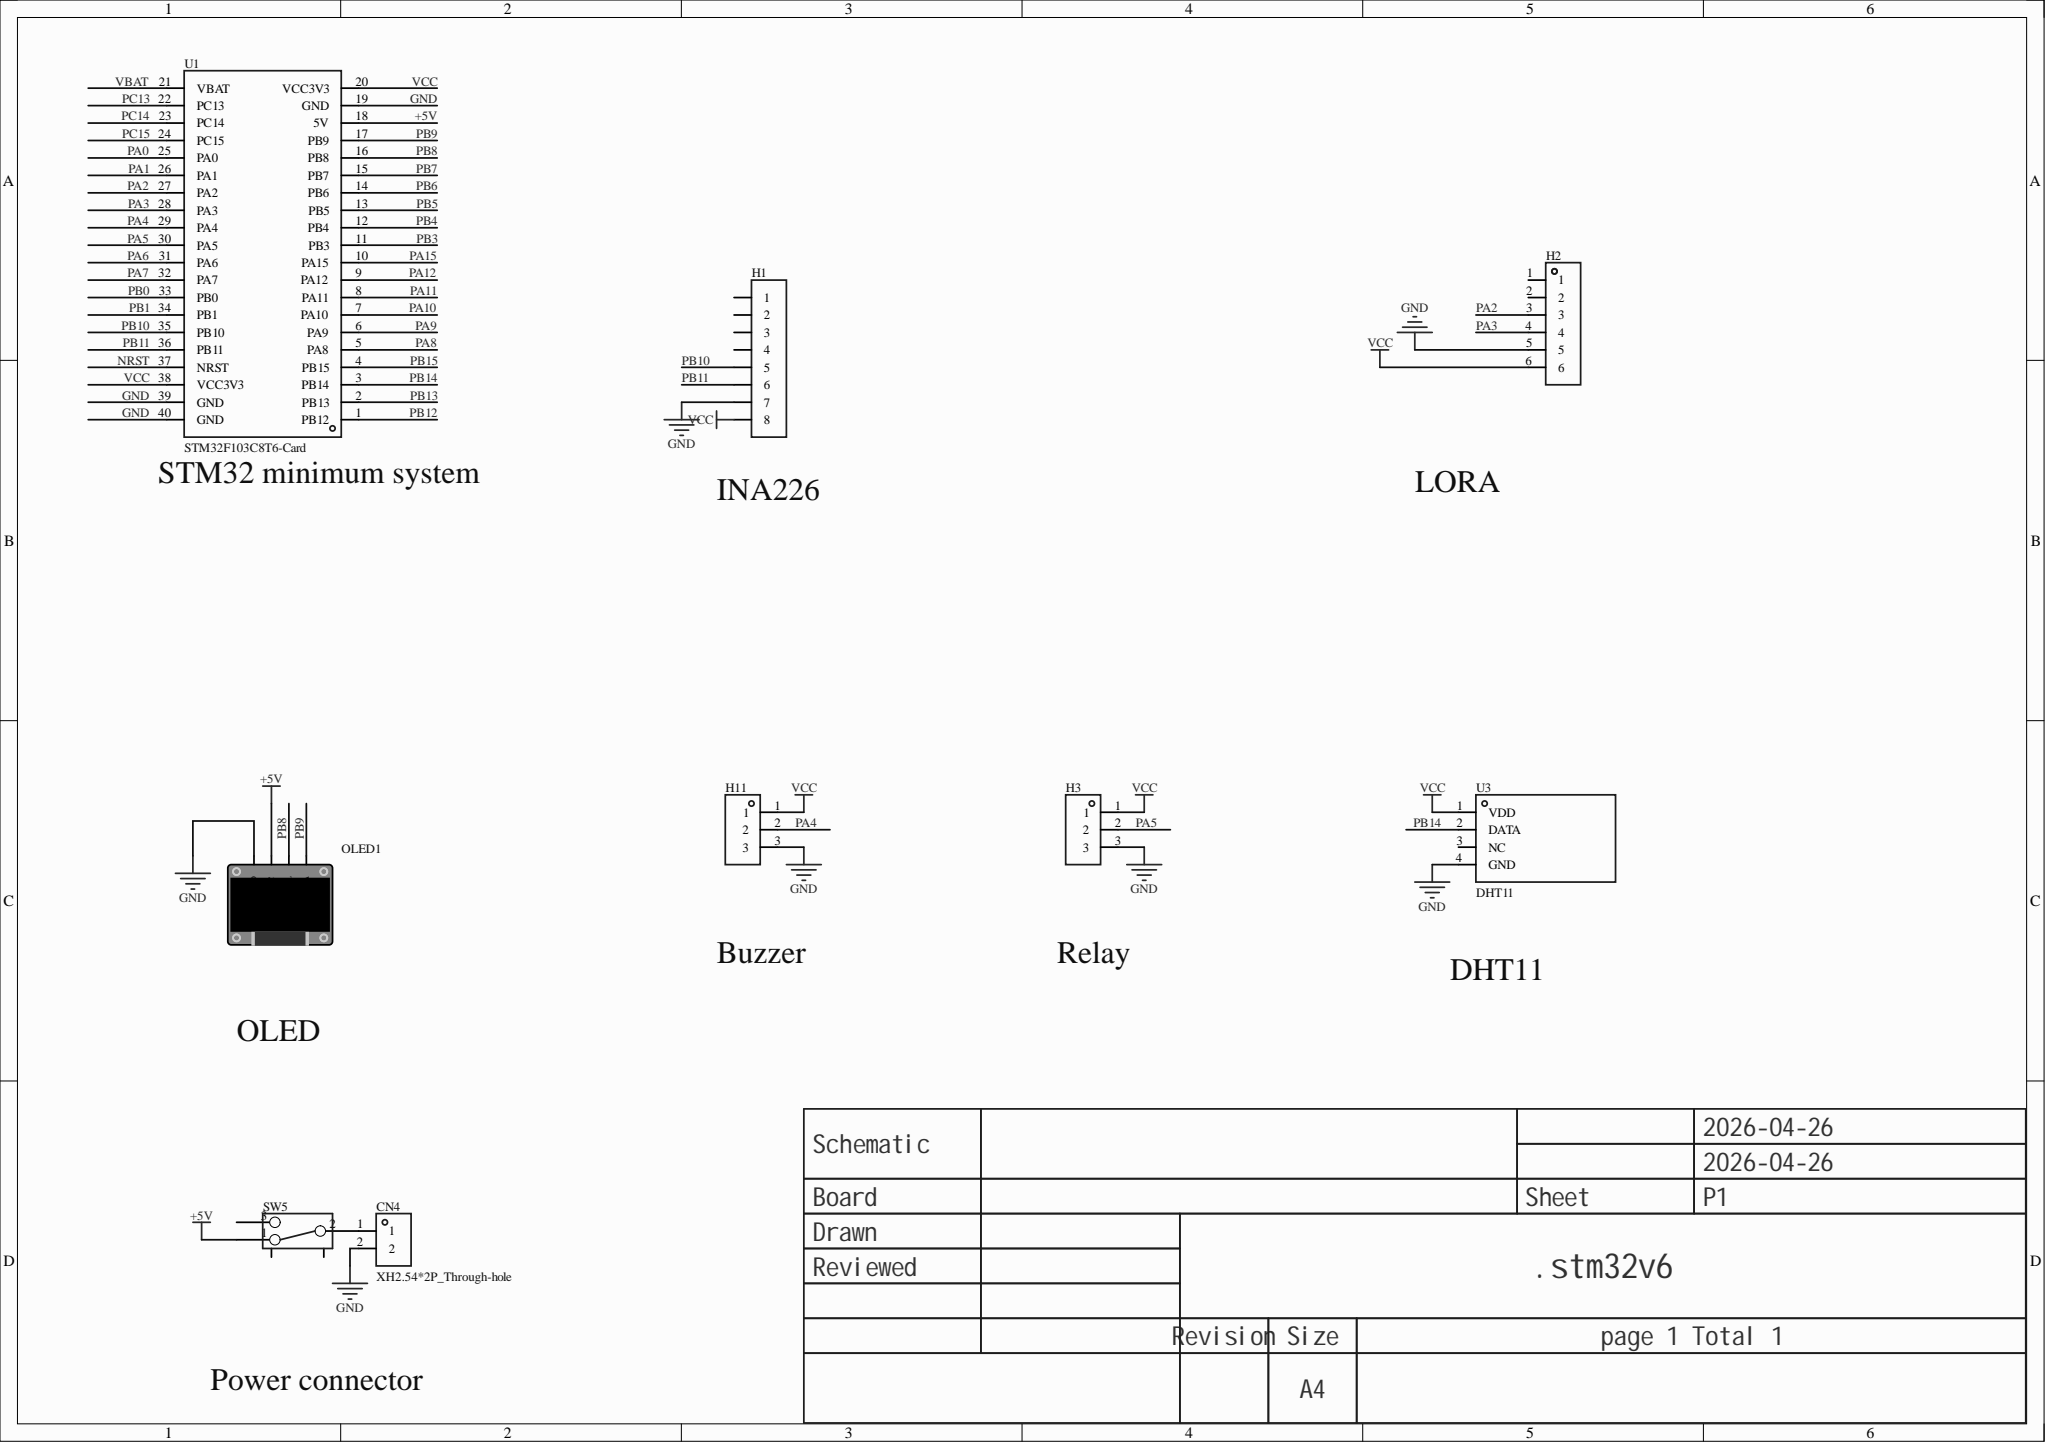Circuit board | Altium Designer | 9 parts | 13 nets
Bill of materials:
Comment,Description,Designator,Footprint,LibRef,Quantity
"XH2.54*2P_Through-hole","","CN4","CONN-TH_2P-P2.50-XH2.54-2P","XH2.54*2P_直插","1"
"","","H1","HDR-TH_8P-P2.54-V-F-1","HDR-F_2.54_1x8P","1"
"","","H2","HDR-TH_6P-P2.54-V-F","HDR-F_2.54_1x6P","1"
"","","H3, H11","HDR-TH_3P-P2.54-V-F","HDR-F_2.54_1x3P","2"
"","","OLED1","0.96OLED_4P","0.96OLED模块_4P","1"
"","","SW5","拨动开关","拨动开关_正","1"
"STM32F103C8T6-Card","","U1","CONN-TH_L53.3-W22.9_STM32F103C8T6-CARD","STM32F103C8T6-Card","1"
"DHT11","New capacitive digital temperature and humidity sensor; old model discontinued 16.1x12.6x5.8mm","U3","SENSOR-TH_DHT11","DHT11","1"
Netlist (Protel format):
[
CN4
CONN-TH_2P-P2.50-XH2.54-2P
XH2.54*2P_Through-hole



]
[
H1
HDR-TH_8P-P2.54-V-F-1




]
[
H2
HDR-TH_6P-P2.54-V-F




]
[
H3
HDR-TH_3P-P2.54-V-F




]
[
H11
HDR-TH_3P-P2.54-V-F




]
[
OLED1
0.96OLED_4P




]
[
SW5
拨动开关




]
[
U1
CONN-TH_L53.3-W22.9_STM32F103C8T6-CARD
STM32F103C8T6-Card



]
[
U3
SENSOR-TH_DHT11
DHT11



]
(
VCC
H1-8
H2-6
H3-1
H11-1
U1-20
U1-38
U3-1
)
(
PB14
U1-3
U3-2
)
(
PB11
H1-6
U1-36
)
(
PB10
H1-5
U1-35
)
(
PB9
OLED1-4
U1-17
)
(
PB8
OLED1-3
U1-16
)
(
PA5
H3-2
U1-30
)
(
PA4
H11-2
U1-29
)
(
PA3
H2-4
U1-28
)
(
PA2
H2-3
U1-27
)
(
NetCN4_1
CN4-1
SW5-2
)
(
GND
CN4-2
H1-7
H2-5
H3-3
H11-3
OLED1-1
U1-19
U1-39
U1-40
U3-4
)
(
+5V
OLED1-2
SW5-1
U1-18
)